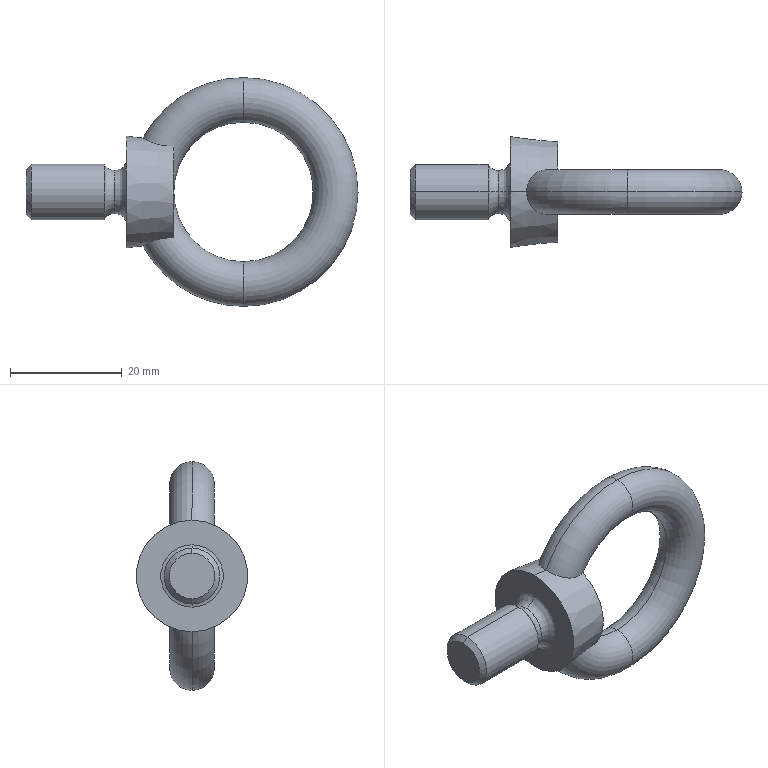Part | STEP file | Eyebolt mounting bracket-Part-2 | 1 solid | 20 faces | box 59.5 x 20 x 41 mm | volume 8069 mm3 | torus 10 | cone 4 | plane 4 | cylinder 2 | commonest cylinder face diameters 10 x2